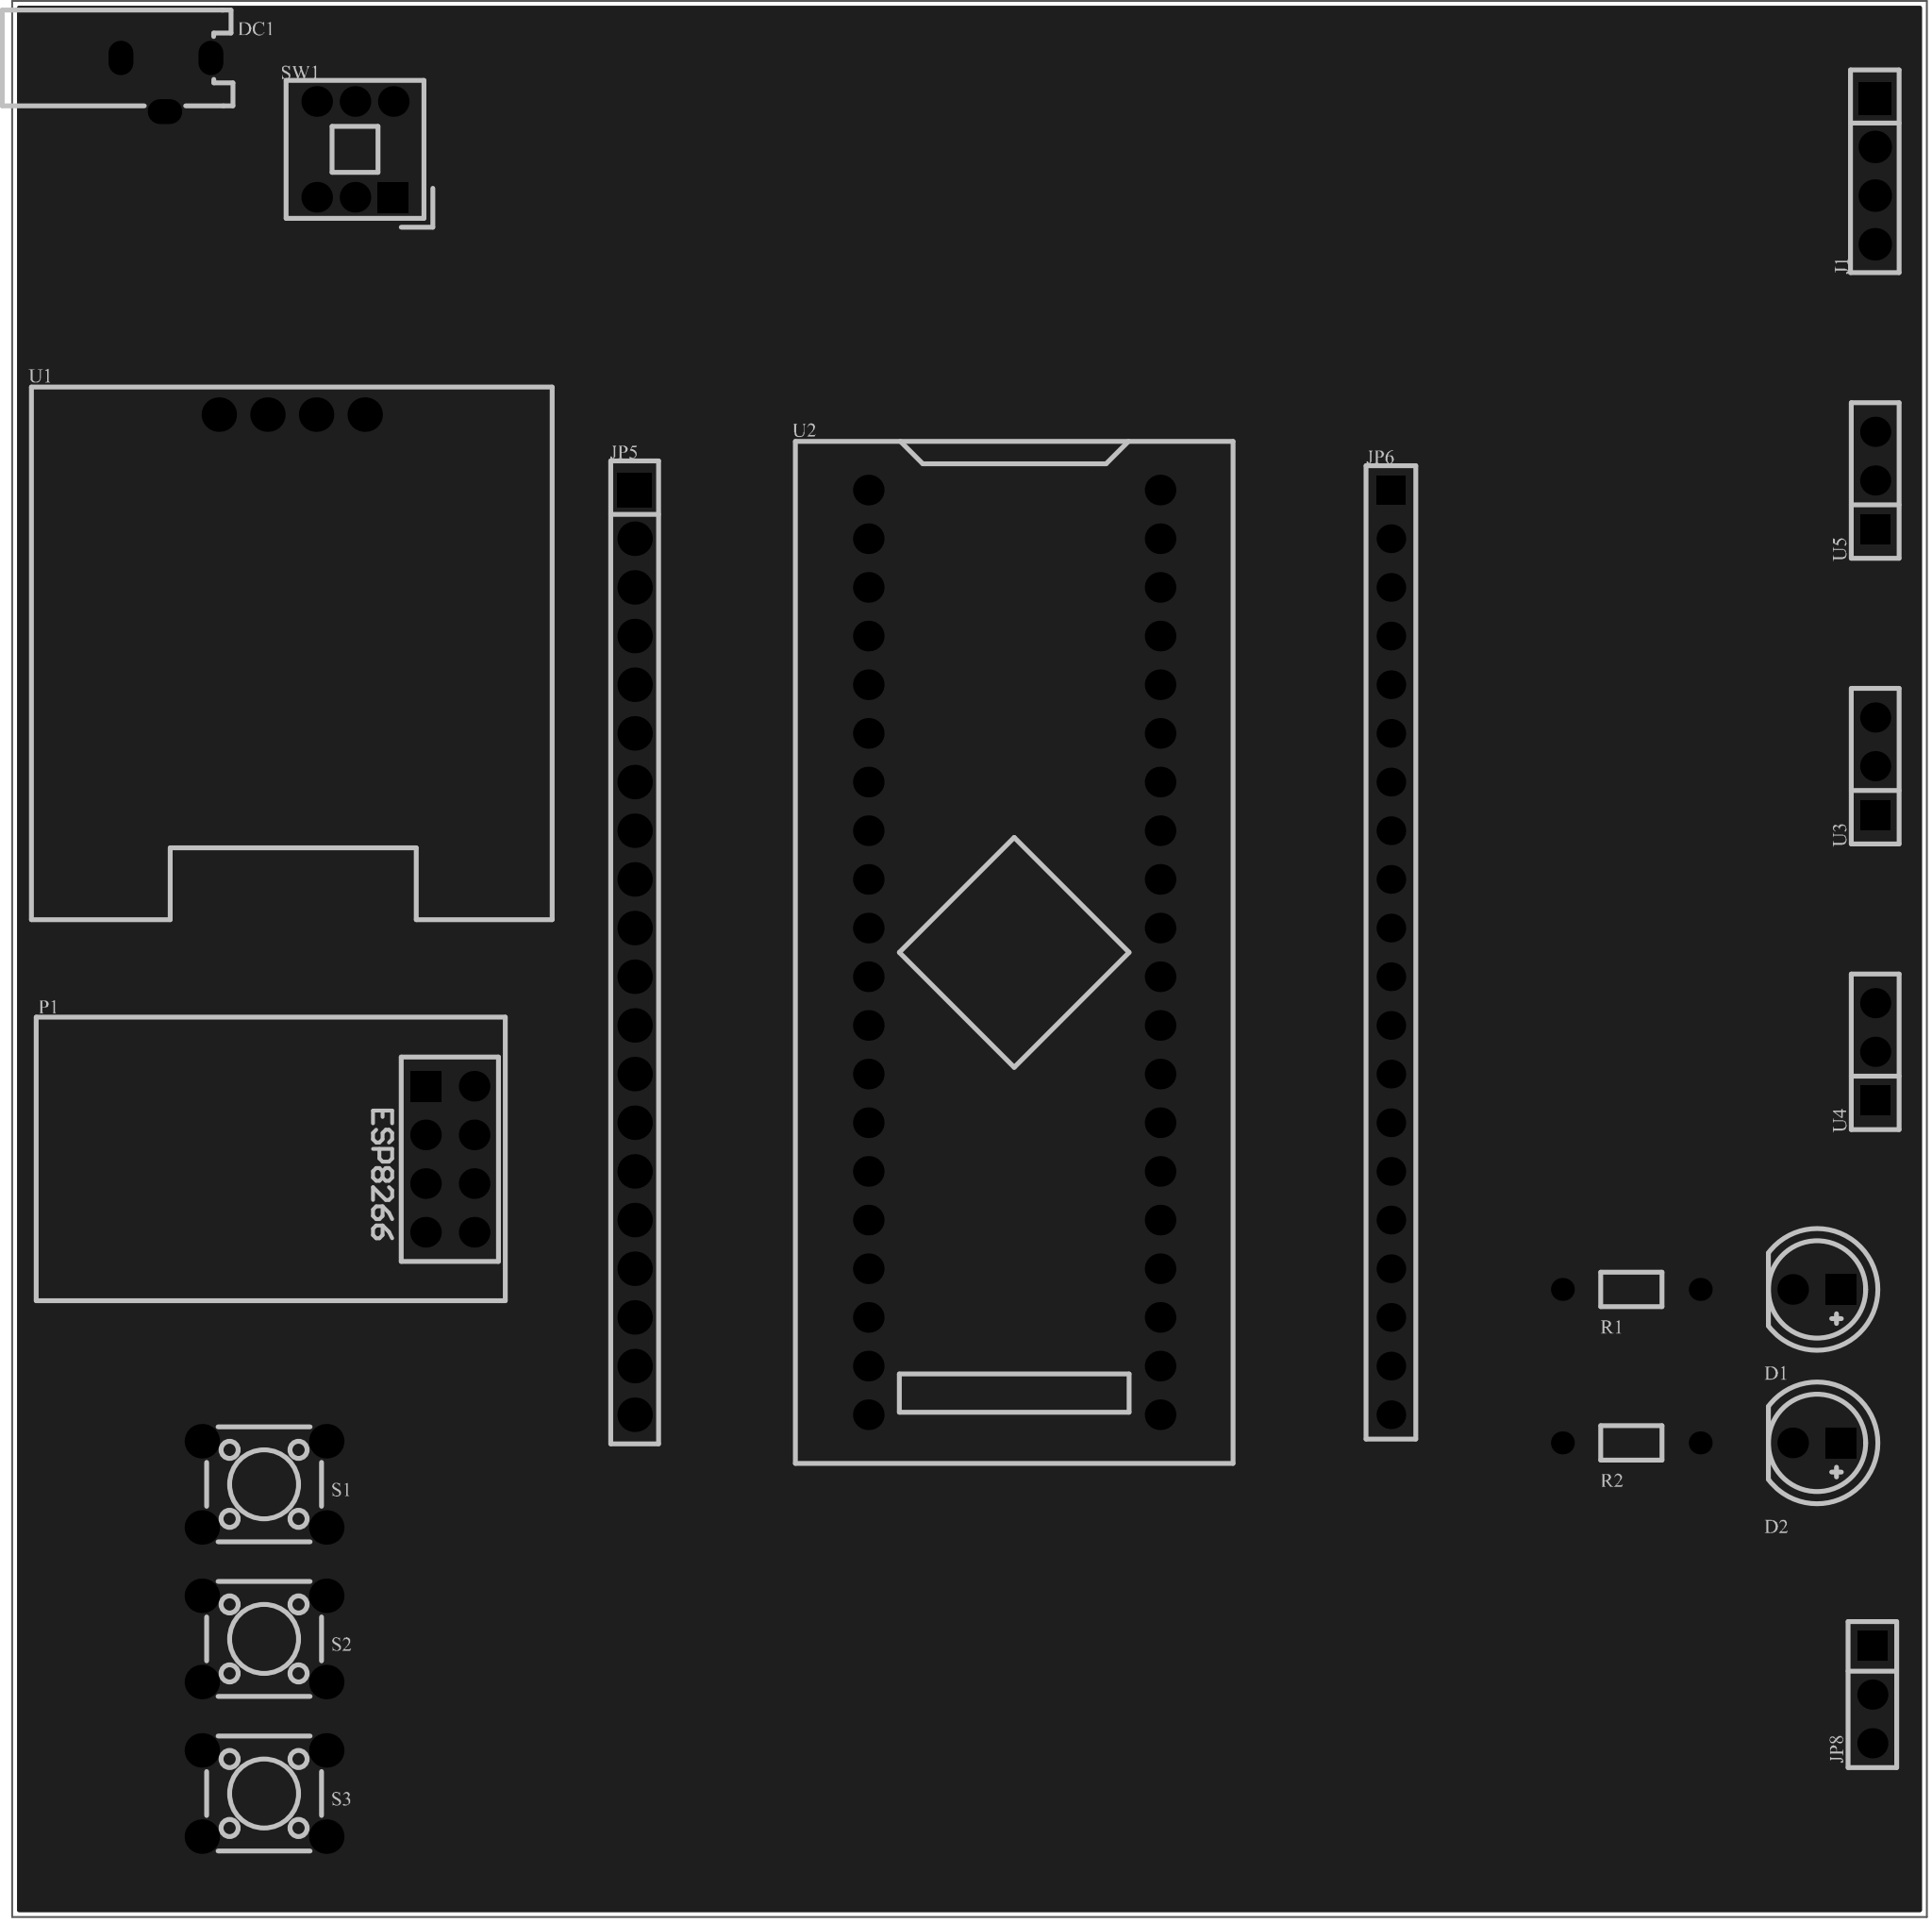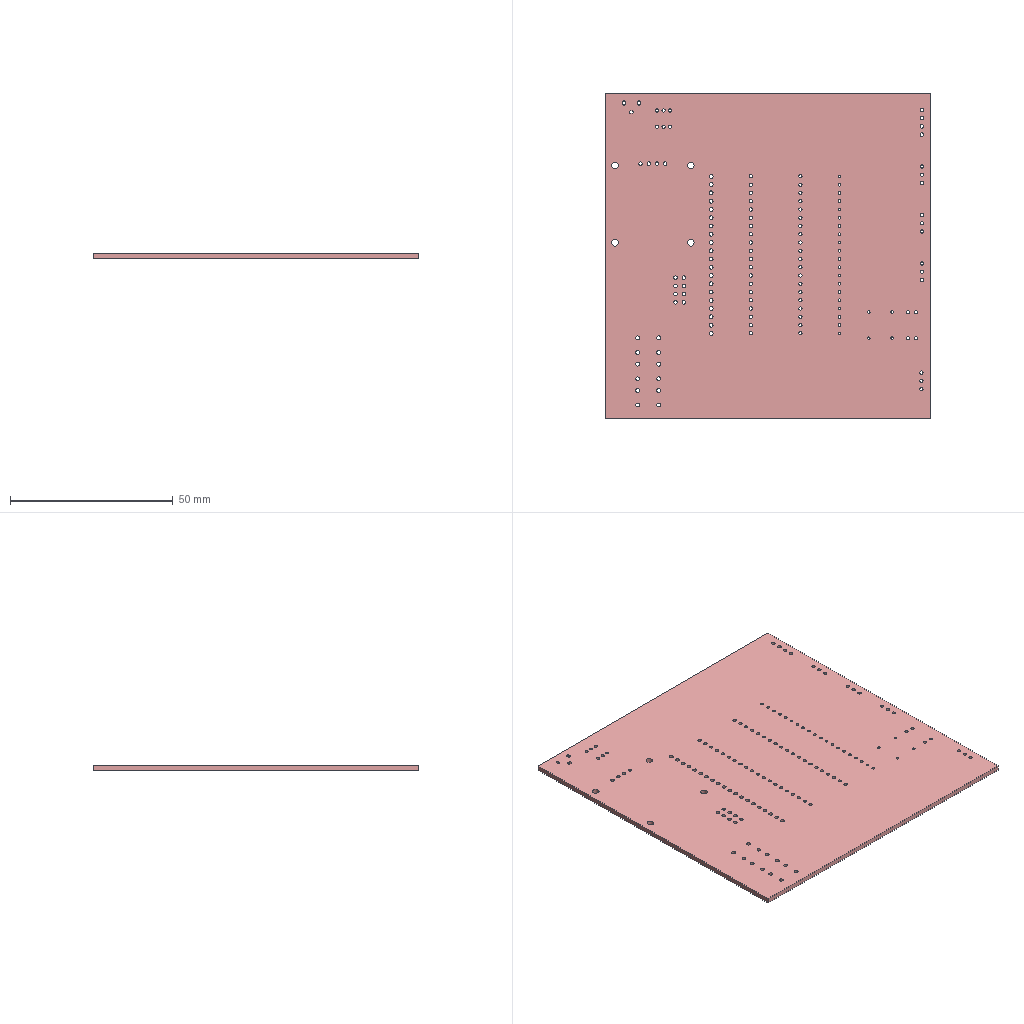Circuit board layout | Altium Designer | box 100 x 100 x 1.6 mm
Layer stack:
# Altium Designer layer stack of  (unit mm; dielectric type: 0 none, 1 core, 2 prepreg, 3 surface material)
index,name,kind,layer,copper_thickness_mm,dielectric_type,dielectric_thickness_mm,dielectric_material,dielectric_constant
0,Top Paste Mask Layer,other,,,,,,
1,Top Silkscreen Layer,other,,,,,,
2,Top Solder Mask Layer,dielectric,,,3,0.01,,3.3
3,Top Layer,copper,Top Layer,0.035,,,,
4,Dielectric1,dielectric,,,3,1.51,FR4,4.5
5,Bottom Layer,copper,Bottom Layer,0.035,,,,
6,Bottom Solder Mask Layer,dielectric,,,3,0.01,,3.3
7,Bottom Silkscreen Layer,other,,,,,,
8,Bottom Paste Mask Layer,other,,,,,,
# drill layer pairs: low layer,high layer
drill_pair,Top Layer,Bottom Layer
Part placement:
Designator,Comment,Layer,Footprint,Center-X(mm),Center-Y(mm),Rotation
D1,led,TopLayer,LED-TH_5mm,187.864,119.571,180
D2,led,TopLayer,LED-TH_5mm,187.864,111.562,180
DC1,DC002-1.3,TopLayer,DC-IN-TH_DC002-1.3,101.631,182.441,270
J1,,TopLayer,HDR-TH_4P-P2.54-V-F,190.881,177.927,270
JP5,HDR-1X20,TopLayer,HDR-TH_20P-P2.54-V-F,126.111,137.16,270
JP6,HDR-1X20,TopLayer,HDR-TH_20P-P2.54-V-F-6,165.608,137.16,270
JP8,HDR-1X3,TopLayer,HDR-TH_3P-P2.54-V-F-4,190.754,98.425,270
P1,,TopLayer,ESP8266-1,116.459,126.365,270
R1,Res2,TopLayer,Res_1/8W,178.166,119.571,180
R2,Res2,TopLayer,Res_1/8W,178.166,111.562,180
S1,key_4,TopLayer,SW-TH_4P-L6.0-W6.0-P4.50-LS6.5,106.757,109.399,180
S2,key_4,TopLayer,SW-TH_4P-L6.0-W6.0-P4.50-LS6.5,106.757,101.331,180
S3,key_4,TopLayer,SW-TH_4P-L6.0-W6.0-P4.50-LS6.5,106.757,93.263,180
SW1,Self-lock button,TopLayer,SW-TH_6P-L7.0-W7.0-P2.00,111.506,179.07,270
U1,OLED,TopLayer,OLED-TH_L27.8-W27.2-P2.54_C9900033791,108.204,165.227,0
U2,ST32F103C8T6,TopLayer,CONN-TH_L53.3-W22.9_STM32F103C8T6-CARD,145.935,137.16,270
U3,,TopLayer,HDR-TH_3P-P2.54-V-F,190.901,146.88,90
U4,,TopLayer,HDR-TH_3P-P2.54-V-F,190.901,131.972,90
U5,DHT11,TopLayer,HDR-TH_3P-P2.54-V-F,190.901,161.788,90
Pad and via stacks:
# Altium Designer via and pad stacks of  (unit mm). Each distinct definition once, with the count of objects using it.
# via: kind,start_layer,end_layer,hole_mm,diameter_mm,mode(0 simple;1 top-mid-bottom;2 full stack),diameter_per_layer,count,example_net
# pad: kind,layer,hole_mm,hole_type(0 round;1 square;2 slot),plating,top_size,top_shape(1 round;2 rect;3 octagon;9 rounded rect),mid_size,bottom_size,mode,footprint,size_per_layer,count,example
pad,Multi-Layer,1,0,plated,1.6x1.6,2,1.6x1.6,1.6x1.6,0,LED-TH_5mm,,2,D1.1
pad,Multi-Layer,1,0,plated,1.6x1.6,1,1.6x1.6,1.6x1.6,0,LED-TH_5mm,,2,D1.2
pad,Multi-Layer,0.8,2,plated,1.3x1.8,1,1.3x1.8,1.3x1.8,0,DC-IN-TH_DC002-1.3,,3,DC1.1
pad,Multi-Layer,1.1,0,plated,1.7x1.7,2,1.7x1.7,1.7x1.7,0,HDR-TH_4P-P2.54-V-F,,1,J1.1
pad,Multi-Layer,1.1,0,plated,1.7x1.7,1,1.7x1.7,1.7x1.7,0,HDR-TH_4P-P2.54-V-F,,3,J1.2
pad,Multi-Layer,1.2,0,plated,1.8x1.8,2,1.8x1.8,1.8x1.8,0,HDR-TH_20P-P2.54-V-F,,1,JP5.1
pad,Multi-Layer,1.2,0,plated,1.8x1.8,1,1.8x1.8,1.8x1.8,0,HDR-TH_20P-P2.54-V-F,,19,JP5.2
pad,Multi-Layer,0.85,0,plated,1.5x1.5,1,1.5x1.5,1.5x1.5,0,HDR-TH_20P-P2.54-V-F-6,,19,JP6.20
pad,Multi-Layer,0.85,0,plated,1.5x1.5,2,1.5x1.5,1.5x1.5,0,HDR-TH_20P-P2.54-V-F-6,,1,JP6.1
pad,Multi-Layer,1.02,0,plated,1.575x1.575,2,1.575x1.575,1.575x1.575,0,HDR-TH_3P-P2.54-V-F-4,,1,JP8.1
pad,Multi-Layer,1.02,0,plated,1.575x1.575,1,1.575x1.575,1.575x1.575,0,HDR-TH_3P-P2.54-V-F-4,,2,JP8.2
pad,Multi-Layer,1.1,0,plated,1.6x1.6,2,1.6x1.6,1.6x1.6,0,ESP8266-1,,1,P1.1
pad,Multi-Layer,1.1,0,plated,1.6x1.6,1,1.6x1.6,1.6x1.6,0,ESP8266-1,,7,P1.2
pad,Multi-Layer,0.8001,0,plated,1.199x1.199,1,1.199x1.199,1.199x1.199,0,Res_1/8W,,4,R1.1
pad,Multi-Layer,1.2,0,plated,1.8x1.8,1,1.8x1.8,1.8x1.8,0,SW-TH_4P-L6.0-W6.0-P4.50-LS6.5,,12,S1.1
pad,Multi-Layer,1,0,plated,1.6x1.6,1,1.6x1.6,1.6x1.6,0,SW-TH_6P-L7.0-W7.0-P2.00,,5,SW1.4
pad,Multi-Layer,1,0,plated,1.6x1.6,2,1.6x1.6,1.6x1.6,0,SW-TH_6P-L7.0-W7.0-P2.00,,1,SW1.1
pad,Multi-Layer,1.05,0,plated,1.8x1.8,1,1.8x1.8,1.8x1.8,0,OLED-TH_L27.8-W27.2-P2.54_C9900033791,,4,U1.1
pad,Multi-Layer,1,0,plated,1.6x1.6,1,1.6x1.6,1.6x1.6,0,CONN-TH_L53.3-W22.9_STM32F103C8T6-CARD,,40,U2.1
pad,Multi-Layer,1.02,0,plated,1.575x1.575,1,1.575x1.575,1.575x1.575,0,HDR-TH_3P-P2.54-V-F,,6,U3.3
pad,Multi-Layer,1.02,0,plated,1.575x1.575,2,1.575x1.575,1.575x1.575,0,HDR-TH_3P-P2.54-V-F,,3,U3.1
Copper pours:
name,layer,net,type(0 solid;1 hatched;2 none)
Top Layer-GND,Top Layer,GND,0
Bottom Layer-GND,Bottom Layer,GND,0